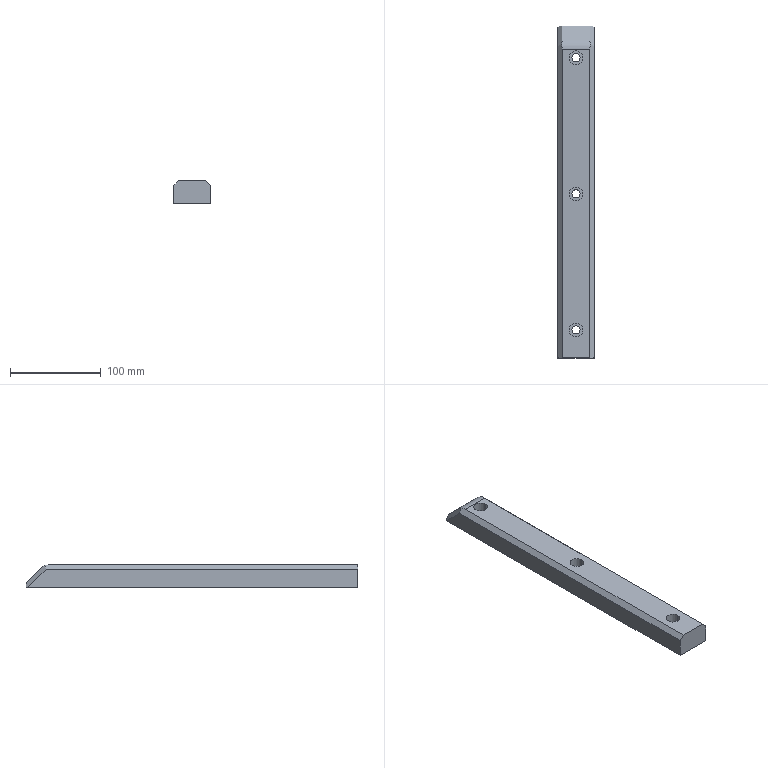Part | SolidWorks | features Chamfer 4, Fillet 4, ICE 3, HoleWzd 2, Extrusion 1 | 1 solid | 27 faces | box 40 x 366 x 25 mm | volume 339646 mm3 | plane 14 | cylinder 13 | commonest cylinder face diameters 9 x6 15 x6 30 x1
STEP:
#1=CARTESIAN_POINT('',(-4.5,-152.,0.));
#2=VERTEX_POINT('',#1);
#3=CARTESIAN_POINT('',(4.5,-152.,0.));
#4=VERTEX_POINT('',#3);
#5=CARTESIAN_POINT('',(0.,-152.,0.));
#6=DIRECTION('',(0.,0.,1.));
#7=DIRECTION('',(1.,0.,0.));
#8=AXIS2_PLACEMENT_3D('',#5,#6,#7);
#9=CIRCLE('',#8,4.5);
#10=EDGE_CURVE('',#2,#4,#9,.T.);
#11=ORIENTED_EDGE('',*,*,#10,.F.);
#12=CARTESIAN_POINT('',(-4.5,-152.,13.));
#13=VERTEX_POINT('',#12);
#14=CARTESIAN_POINT('',(-4.5,-152.,23.));
#15=DIRECTION('',(0.,0.,1.));
#16=VECTOR('',#15,1000.);
#17=LINE('',#14,#16);
#18=EDGE_CURVE('',#2,#13,#17,.T.);
#19=ORIENTED_EDGE('',*,*,#18,.T.);
#20=CARTESIAN_POINT('',(4.5,-152.,13.));
#21=VERTEX_POINT('',#20);
#22=CARTESIAN_POINT('',(0.,-152.,13.));
#23=DIRECTION('',(0.,0.,1.));
#24=DIRECTION('',(1.,0.,0.));
#25=AXIS2_PLACEMENT_3D('',#22,#23,#24);
#26=CIRCLE('',#25,4.5);
#27=EDGE_CURVE('',#13,#21,#26,.T.);
#28=ORIENTED_EDGE('',*,*,#27,.T.);
#29=CARTESIAN_POINT('',(4.5,-152.,23.));
#30=DIRECTION('',(0.,0.,1.));
#31=VECTOR('',#30,1000.);
#32=LINE('',#29,#31);
#33=EDGE_CURVE('',#4,#21,#32,.T.);
#34=ORIENTED_EDGE('',*,*,#33,.F.);
#35=EDGE_LOOP('',(#11,#19,#28,#34));
#36=FACE_OUTER_BOUND('',#35,.T.);
#37=CARTESIAN_POINT('',(0.,-152.,23.));
#38=DIRECTION('',(0.,0.,1.));
#39=DIRECTION('',(1.,0.,0.));
#40=AXIS2_PLACEMENT_3D('',#37,#38,#39);
#41=CYLINDRICAL_SURFACE('',#40,4.5);
#42=ADVANCED_FACE('',(#36),#41,.F.);
#43=CARTESIAN_POINT('',(-4.5,-2.,0.));
#44=VERTEX_POINT('',#43);
#45=CARTESIAN_POINT('',(4.5,-2.,0.));
#46=VERTEX_POINT('',#45);
#47=CARTESIAN_POINT('',(0.,-2.,0.));
#48=DIRECTION('',(0.,0.,1.));
#49=DIRECTION('',(1.,0.,0.));
#50=AXIS2_PLACEMENT_3D('',#47,#48,#49);
#51=CIRCLE('',#50,4.5);
#52=EDGE_CURVE('',#44,#46,#51,.T.);
#53=ORIENTED_EDGE('',*,*,#52,.F.);
#54=CARTESIAN_POINT('',(-4.5,-2.,13.));
#55=VERTEX_POINT('',#54);
#56=CARTESIAN_POINT('',(-4.5,-2.,23.));
#57=DIRECTION('',(0.,0.,1.));
#58=VECTOR('',#57,1000.);
#59=LINE('',#56,#58);
#60=EDGE_CURVE('',#44,#55,#59,.T.);
#61=ORIENTED_EDGE('',*,*,#60,.T.);
#62=CARTESIAN_POINT('',(4.5,-2.,13.));
#63=VERTEX_POINT('',#62);
#64=CARTESIAN_POINT('',(0.,-2.,13.));
#65=DIRECTION('',(0.,0.,1.));
#66=DIRECTION('',(1.,0.,0.));
#67=AXIS2_PLACEMENT_3D('',#64,#65,#66);
#68=CIRCLE('',#67,4.5);
#69=EDGE_CURVE('',#55,#63,#68,.T.);
#70=ORIENTED_EDGE('',*,*,#69,.T.);
#71=CARTESIAN_POINT('',(4.5,-2.,23.));
#72=DIRECTION('',(0.,0.,1.));
#73=VECTOR('',#72,1000.);
#74=LINE('',#71,#73);
#75=EDGE_CURVE('',#46,#63,#74,.T.);
#76=ORIENTED_EDGE('',*,*,#75,.F.);
#77=EDGE_LOOP('',(#53,#61,#70,#76));
#78=FACE_OUTER_BOUND('',#77,.T.);
#79=CARTESIAN_POINT('',(0.,-2.,23.));
#80=DIRECTION('',(0.,0.,1.));
#81=DIRECTION('',(1.,0.,0.));
#82=AXIS2_PLACEMENT_3D('',#79,#80,#81);
#83=CYLINDRICAL_SURFACE('',#82,4.5);
#84=ADVANCED_FACE('',(#78),#83,.F.);
#85=CARTESIAN_POINT('',(-4.5,148.,0.));
#86=VERTEX_POINT('',#85);
#87=CARTESIAN_POINT('',(4.5,148.,0.));
#88=VERTEX_POINT('',#87);
#89=CARTESIAN_POINT('',(0.,148.,0.));
#90=DIRECTION('',(0.,0.,1.));
#91=DIRECTION('',(1.,0.,0.));
#92=AXIS2_PLACEMENT_3D('',#89,#90,#91);
#93=CIRCLE('',#92,4.5);
#94=EDGE_CURVE('',#86,#88,#93,.T.);
#95=ORIENTED_EDGE('',*,*,#94,.F.);
#96=CARTESIAN_POINT('',(-4.5,148.,13.));
#97=VERTEX_POINT('',#96);
#98=CARTESIAN_POINT('',(-4.5,148.,23.));
#99=DIRECTION('',(0.,0.,1.));
#100=VECTOR('',#99,1000.);
#101=LINE('',#98,#100);
#102=EDGE_CURVE('',#86,#97,#101,.T.);
#103=ORIENTED_EDGE('',*,*,#102,.T.);
#104=CARTESIAN_POINT('',(4.5,148.,13.));
#105=VERTEX_POINT('',#104);
#106=CARTESIAN_POINT('',(0.,148.,13.));
#107=DIRECTION('',(0.,0.,1.));
#108=DIRECTION('',(1.,0.,0.));
#109=AXIS2_PLACEMENT_3D('',#106,#107,#108);
#110=CIRCLE('',#109,4.5);
#111=EDGE_CURVE('',#97,#105,#110,.T.);
#112=ORIENTED_EDGE('',*,*,#111,.T.);
#113=CARTESIAN_POINT('',(4.5,148.,23.));
#114=DIRECTION('',(0.,0.,1.));
#115=VECTOR('',#114,1000.);
#116=LINE('',#113,#115);
#117=EDGE_CURVE('',#88,#105,#116,.T.);
#118=ORIENTED_EDGE('',*,*,#117,.F.);
#119=EDGE_LOOP('',(#95,#103,#112,#118));
#120=FACE_OUTER_BOUND('',#119,.T.);
#121=CARTESIAN_POINT('',(0.,148.,23.));
#122=DIRECTION('',(0.,0.,1.));
#123=DIRECTION('',(1.,0.,0.));
#124=AXIS2_PLACEMENT_3D('',#121,#122,#123);
#125=CYLINDRICAL_SURFACE('',#124,4.5);
#126=ADVANCED_FACE('',(#120),#125,.F.);
#127=CARTESIAN_POINT('',(-7.5,-152.,13.));
#128=VERTEX_POINT('',#127);
#129=CARTESIAN_POINT('',(7.5,-152.,13.));
#130=VERTEX_POINT('',#129);
#131=CARTESIAN_POINT('',(0.,-152.,13.));
#132=DIRECTION('',(0.,0.,1.));
#133=DIRECTION('',(1.,0.,0.));
#134=AXIS2_PLACEMENT_3D('',#131,#132,#133);
#135=CIRCLE('',#134,7.5);
#136=EDGE_CURVE('',#128,#130,#135,.T.);
#137=ORIENTED_EDGE('',*,*,#136,.F.);
#138=CARTESIAN_POINT('',(-7.5,-152.,25.));
#139=VERTEX_POINT('',#138);
#140=CARTESIAN_POINT('',(-7.5,-152.,23.));
#141=DIRECTION('',(0.,0.,1.));
#142=VECTOR('',#141,1000.);
#143=LINE('',#140,#142);
#144=EDGE_CURVE('',#128,#139,#143,.T.);
#145=ORIENTED_EDGE('',*,*,#144,.T.);
#146=CARTESIAN_POINT('',(7.5,-152.,25.));
#147=VERTEX_POINT('',#146);
#148=CARTESIAN_POINT('',(0.,-152.,25.));
#149=DIRECTION('',(0.,0.,1.));
#150=DIRECTION('',(1.,0.,0.));
#151=AXIS2_PLACEMENT_3D('',#148,#149,#150);
#152=CIRCLE('',#151,7.5);
#153=EDGE_CURVE('',#139,#147,#152,.T.);
#154=ORIENTED_EDGE('',*,*,#153,.T.);
#155=CARTESIAN_POINT('',(7.5,-152.,23.));
#156=DIRECTION('',(0.,0.,1.));
#157=VECTOR('',#156,1000.);
#158=LINE('',#155,#157);
#159=EDGE_CURVE('',#130,#147,#158,.T.);
#160=ORIENTED_EDGE('',*,*,#159,.F.);
#161=EDGE_LOOP('',(#137,#145,#154,#160));
#162=FACE_OUTER_BOUND('',#161,.T.);
#163=CARTESIAN_POINT('',(0.,-152.,23.));
#164=DIRECTION('',(0.,0.,1.));
#165=DIRECTION('',(1.,0.,0.));
#166=AXIS2_PLACEMENT_3D('',#163,#164,#165);
#167=CYLINDRICAL_SURFACE('',#166,7.5);
#168=ADVANCED_FACE('',(#162),#167,.F.);
#169=CARTESIAN_POINT('',(-7.5,-2.,13.));
#170=VERTEX_POINT('',#169);
#171=CARTESIAN_POINT('',(7.5,-2.,13.));
#172=VERTEX_POINT('',#171);
#173=CARTESIAN_POINT('',(0.,-2.,13.));
#174=DIRECTION('',(0.,0.,1.));
#175=DIRECTION('',(1.,0.,0.));
#176=AXIS2_PLACEMENT_3D('',#173,#174,#175);
#177=CIRCLE('',#176,7.5);
#178=EDGE_CURVE('',#170,#172,#177,.T.);
#179=ORIENTED_EDGE('',*,*,#178,.F.);
#180=CARTESIAN_POINT('',(-7.5,-2.,25.));
#181=VERTEX_POINT('',#180);
#182=CARTESIAN_POINT('',(-7.5,-2.,23.));
#183=DIRECTION('',(0.,0.,1.));
#184=VECTOR('',#183,1000.);
#185=LINE('',#182,#184);
#186=EDGE_CURVE('',#170,#181,#185,.T.);
#187=ORIENTED_EDGE('',*,*,#186,.T.);
#188=CARTESIAN_POINT('',(7.5,-2.,25.));
#189=VERTEX_POINT('',#188);
#190=CARTESIAN_POINT('',(0.,-2.,25.));
#191=DIRECTION('',(0.,0.,1.));
#192=DIRECTION('',(1.,0.,0.));
#193=AXIS2_PLACEMENT_3D('',#190,#191,#192);
#194=CIRCLE('',#193,7.5);
#195=EDGE_CURVE('',#181,#189,#194,.T.);
#196=ORIENTED_EDGE('',*,*,#195,.T.);
#197=CARTESIAN_POINT('',(7.5,-2.,23.));
#198=DIRECTION('',(0.,0.,1.));
#199=VECTOR('',#198,1000.);
#200=LINE('',#197,#199);
#201=EDGE_CURVE('',#172,#189,#200,.T.);
#202=ORIENTED_EDGE('',*,*,#201,.F.);
#203=EDGE_LOOP('',(#179,#187,#196,#202));
#204=FACE_OUTER_BOUND('',#203,.T.);
#205=CARTESIAN_POINT('',(0.,-2.,23.));
#206=DIRECTION('',(0.,0.,1.));
#207=DIRECTION('',(1.,0.,0.));
#208=AXIS2_PLACEMENT_3D('',#205,#206,#207);
#209=CYLINDRICAL_SURFACE('',#208,7.5);
#210=ADVANCED_FACE('',(#204),#209,.F.);
#211=CARTESIAN_POINT('',(-7.5,148.,13.));
#212=VERTEX_POINT('',#211);
#213=CARTESIAN_POINT('',(7.5,148.,13.));
#214=VERTEX_POINT('',#213);
#215=CARTESIAN_POINT('',(0.,148.,13.));
#216=DIRECTION('',(0.,0.,1.));
#217=DIRECTION('',(1.,0.,0.));
#218=AXIS2_PLACEMENT_3D('',#215,#216,#217);
#219=CIRCLE('',#218,7.5);
#220=EDGE_CURVE('',#212,#214,#219,.T.);
#221=ORIENTED_EDGE('',*,*,#220,.F.);
#222=CARTESIAN_POINT('',(-7.5,148.,25.));
#223=VERTEX_POINT('',#222);
#224=CARTESIAN_POINT('',(-7.5,148.,23.));
#225=DIRECTION('',(0.,0.,1.));
#226=VECTOR('',#225,1000.);
#227=LINE('',#224,#226);
#228=EDGE_CURVE('',#212,#223,#227,.T.);
#229=ORIENTED_EDGE('',*,*,#228,.T.);
#230=CARTESIAN_POINT('',(7.5,148.,25.));
#231=VERTEX_POINT('',#230);
#232=CARTESIAN_POINT('',(0.,148.,25.));
#233=DIRECTION('',(0.,0.,1.));
#234=DIRECTION('',(1.,0.,0.));
#235=AXIS2_PLACEMENT_3D('',#232,#233,#234);
#236=CIRCLE('',#235,7.5);
#237=EDGE_CURVE('',#223,#231,#236,.T.);
#238=ORIENTED_EDGE('',*,*,#237,.T.);
#239=CARTESIAN_POINT('',(7.5,148.,23.));
#240=DIRECTION('',(0.,0.,1.));
#241=VECTOR('',#240,1000.);
#242=LINE('',#239,#241);
#243=EDGE_CURVE('',#214,#231,#242,.T.);
#244=ORIENTED_EDGE('',*,*,#243,.F.);
#245=EDGE_LOOP('',(#221,#229,#238,#244));
#246=FACE_OUTER_BOUND('',#245,.T.);
#247=CARTESIAN_POINT('',(0.,148.,23.));
#248=DIRECTION('',(0.,0.,1.));
#249=DIRECTION('',(1.,0.,0.));
#250=AXIS2_PLACEMENT_3D('',#247,#248,#249);
#251=CYLINDRICAL_SURFACE('',#250,7.5);
#252=ADVANCED_FACE('',(#246),#251,.F.);
#253=CARTESIAN_POINT('',(20.,-183.,0.));
#254=VERTEX_POINT('',#253);
#255=CARTESIAN_POINT('',(20.,180.929,0.));
#256=VERTEX_POINT('',#255);
#257=CARTESIAN_POINT('',(20.,183.,0.));
#258=DIRECTION('',(0.,1.,0.));
#259=VECTOR('',#258,1000.);
#260=LINE('',#257,#259);
#261=EDGE_CURVE('',#254,#256,#260,.T.);
#262=ORIENTED_EDGE('',*,*,#261,.T.);
#263=CARTESIAN_POINT('',(20.,160.929,20.));
#264=VERTEX_POINT('',#263);
#265=CARTESIAN_POINT('',(20.,164.464,16.464));
#266=DIRECTION('',(0.,-0.7071,0.7071));
#267=VECTOR('',#266,1000.);
#268=LINE('',#265,#267);
#269=EDGE_CURVE('',#256,#264,#268,.T.);
#270=ORIENTED_EDGE('',*,*,#269,.T.);
#271=CARTESIAN_POINT('',(20.,-183.,20.));
#272=VERTEX_POINT('',#271);
#273=CARTESIAN_POINT('',(20.,-183.,20.));
#274=DIRECTION('',(0.,-1.,0.));
#275=VECTOR('',#274,1000.);
#276=LINE('',#273,#275);
#277=EDGE_CURVE('',#264,#272,#276,.T.);
#278=ORIENTED_EDGE('',*,*,#277,.T.);
#279=CARTESIAN_POINT('',(20.,-183.,25.));
#280=DIRECTION('',(0.,0.,-1.));
#281=VECTOR('',#280,1000.);
#282=LINE('',#279,#281);
#283=EDGE_CURVE('',#272,#254,#282,.T.);
#284=ORIENTED_EDGE('',*,*,#283,.T.);
#285=EDGE_LOOP('',(#262,#270,#278,#284));
#286=FACE_OUTER_BOUND('',#285,.T.);
#287=CARTESIAN_POINT('',(20.,183.,25.));
#288=DIRECTION('',(-1.,0.,0.));
#289=DIRECTION('',(0.,-1.,0.));
#290=AXIS2_PLACEMENT_3D('',#287,#288,#289);
#291=PLANE('',#290);
#292=ADVANCED_FACE('',(#286),#291,.F.);
#293=CARTESIAN_POINT('',(-15.,183.,5.));
#294=VERTEX_POINT('',#293);
#295=CARTESIAN_POINT('',(15.,183.,5.));
#296=VERTEX_POINT('',#295);
#297=CARTESIAN_POINT('',(20.,183.,5.));
#298=DIRECTION('',(1.,0.,0.));
#299=VECTOR('',#298,1000.);
#300=LINE('',#297,#299);
#301=EDGE_CURVE('',#294,#296,#300,.T.);
#302=ORIENTED_EDGE('',*,*,#301,.T.);
#303=CARTESIAN_POINT('',(18.536,183.,0.));
#304=VERTEX_POINT('',#303);
#305=CARTESIAN_POINT('',(13.619,183.,6.953));
#306=DIRECTION('',(0.5774,0.,-0.8165));
#307=VECTOR('',#306,1000.);
#308=LINE('',#305,#307);
#309=EDGE_CURVE('',#296,#304,#308,.T.);
#310=ORIENTED_EDGE('',*,*,#309,.T.);
#311=CARTESIAN_POINT('',(-18.536,183.,0.));
#312=VERTEX_POINT('',#311);
#313=CARTESIAN_POINT('',(-20.,183.,0.));
#314=DIRECTION('',(-1.,0.,0.));
#315=VECTOR('',#314,1000.);
#316=LINE('',#313,#315);
#317=EDGE_CURVE('',#304,#312,#316,.T.);
#318=ORIENTED_EDGE('',*,*,#317,.T.);
#319=CARTESIAN_POINT('',(-13.619,183.,6.953));
#320=DIRECTION('',(0.5774,0.,0.8165));
#321=VECTOR('',#320,1000.);
#322=LINE('',#319,#321);
#323=EDGE_CURVE('',#312,#294,#322,.T.);
#324=ORIENTED_EDGE('',*,*,#323,.T.);
#325=EDGE_LOOP('',(#302,#310,#318,#324));
#326=FACE_OUTER_BOUND('',#325,.T.);
#327=CARTESIAN_POINT('',(-20.,183.,25.));
#328=DIRECTION('',(0.,-1.,0.));
#329=DIRECTION('',(0.,0.,-1.));
#330=AXIS2_PLACEMENT_3D('',#327,#328,#329);
#331=PLANE('',#330);
#332=ADVANCED_FACE('',(#326),#331,.F.);
#333=CARTESIAN_POINT('',(-20.,-183.,20.));
#334=VERTEX_POINT('',#333);
#335=CARTESIAN_POINT('',(-20.,160.929,20.));
#336=VERTEX_POINT('',#335);
#337=CARTESIAN_POINT('',(-20.,163.,20.));
#338=DIRECTION('',(0.,1.,0.));
#339=VECTOR('',#338,1000.);
#340=LINE('',#337,#339);
#341=EDGE_CURVE('',#334,#336,#340,.T.);
#342=ORIENTED_EDGE('',*,*,#341,.T.);
#343=CARTESIAN_POINT('',(-20.,180.929,0.));
#344=VERTEX_POINT('',#343);
#345=CARTESIAN_POINT('',(-20.,179.464,1.464));
#346=DIRECTION('',(0.,0.7071,-0.7071));
#347=VECTOR('',#346,1000.);
#348=LINE('',#345,#347);
#349=EDGE_CURVE('',#336,#344,#348,.T.);
#350=ORIENTED_EDGE('',*,*,#349,.T.);
#351=CARTESIAN_POINT('',(-20.,-183.,0.));
#352=VERTEX_POINT('',#351);
#353=CARTESIAN_POINT('',(-20.,183.,0.));
#354=DIRECTION('',(0.,-1.,0.));
#355=VECTOR('',#354,1000.);
#356=LINE('',#353,#355);
#357=EDGE_CURVE('',#344,#352,#356,.T.);
#358=ORIENTED_EDGE('',*,*,#357,.T.);
#359=CARTESIAN_POINT('',(-20.,-183.,25.));
#360=DIRECTION('',(0.,0.,-1.));
#361=VECTOR('',#360,1000.);
#362=LINE('',#359,#361);
#363=EDGE_CURVE('',#334,#352,#362,.T.);
#364=ORIENTED_EDGE('',*,*,#363,.F.);
#365=EDGE_LOOP('',(#342,#350,#358,#364));
#366=FACE_OUTER_BOUND('',#365,.T.);
#367=CARTESIAN_POINT('',(-20.,183.,25.));
#368=DIRECTION('',(1.,0.,0.));
#369=DIRECTION('',(0.,1.,0.));
#370=AXIS2_PLACEMENT_3D('',#367,#368,#369);
#371=PLANE('',#370);
#372=ADVANCED_FACE('',(#366),#371,.F.);
#373=ORIENTED_EDGE('',*,*,#283,.F.);
#374=CARTESIAN_POINT('',(15.,-183.,25.));
#375=VERTEX_POINT('',#374);
#376=CARTESIAN_POINT('',(15.,-183.,25.));
#377=DIRECTION('',(-0.7071,0.,0.7071));
#378=VECTOR('',#377,1000.);
#379=LINE('',#376,#378);
#380=EDGE_CURVE('',#272,#375,#379,.T.);
#381=ORIENTED_EDGE('',*,*,#380,.T.);
#382=CARTESIAN_POINT('',(-15.,-183.,25.));
#383=VERTEX_POINT('',#382);
#384=CARTESIAN_POINT('',(-20.,-183.,25.));
#385=DIRECTION('',(1.,0.,0.));
#386=VECTOR('',#385,1000.);
#387=LINE('',#384,#386);
#388=EDGE_CURVE('',#383,#375,#387,.T.);
#389=ORIENTED_EDGE('',*,*,#388,.F.);
#390=CARTESIAN_POINT('',(-15.,-183.,25.));
#391=DIRECTION('',(-0.7071,0.,-0.7071));
#392=VECTOR('',#391,1000.);
#393=LINE('',#390,#392);
#394=EDGE_CURVE('',#383,#334,#393,.T.);
#395=ORIENTED_EDGE('',*,*,#394,.T.);
#396=ORIENTED_EDGE('',*,*,#363,.T.);
#397=CARTESIAN_POINT('',(-20.,-183.,0.));
#398=DIRECTION('',(1.,0.,0.));
#399=VECTOR('',#398,1000.);
#400=LINE('',#397,#399);
#401=EDGE_CURVE('',#352,#254,#400,.T.);
#402=ORIENTED_EDGE('',*,*,#401,.T.);
#403=EDGE_LOOP('',(#373,#381,#389,#395,#396,#402));
#404=FACE_OUTER_BOUND('',#403,.T.);
#405=CARTESIAN_POINT('',(-20.,-183.,25.));
#406=DIRECTION('',(0.,1.,0.));
#407=DIRECTION('',(0.,0.,1.));
#408=AXIS2_PLACEMENT_3D('',#405,#406,#407);
#409=PLANE('',#408);
#410=ADVANCED_FACE('',(#404),#409,.F.);
#411=CARTESIAN_POINT('',(0.,-152.,25.));
#412=DIRECTION('',(0.,0.,1.));
#413=DIRECTION('',(1.,0.,0.));
#414=AXIS2_PLACEMENT_3D('',#411,#412,#413);
#415=CIRCLE('',#414,7.5);
#416=EDGE_CURVE('',#147,#139,#415,.T.);
#417=ORIENTED_EDGE('',*,*,#416,.F.);
#418=ORIENTED_EDGE('',*,*,#153,.F.);
#419=EDGE_LOOP('',(#417,#418));
#420=FACE_BOUND('',#419,.T.);
#421=CARTESIAN_POINT('',(0.,-2.,25.));
#422=DIRECTION('',(0.,0.,1.));
#423=DIRECTION('',(1.,0.,0.));
#424=AXIS2_PLACEMENT_3D('',#421,#422,#423);
#425=CIRCLE('',#424,7.5);
#426=EDGE_CURVE('',#189,#181,#425,.T.);
#427=ORIENTED_EDGE('',*,*,#426,.F.);
#428=ORIENTED_EDGE('',*,*,#195,.F.);
#429=EDGE_LOOP('',(#427,#428));
#430=FACE_BOUND('',#429,.T.);
#431=CARTESIAN_POINT('',(0.,148.,25.));
#432=DIRECTION('',(0.,0.,1.));
#433=DIRECTION('',(1.,0.,0.));
#434=AXIS2_PLACEMENT_3D('',#431,#432,#433);
#435=CIRCLE('',#434,7.5);
#436=EDGE_CURVE('',#231,#223,#435,.T.);
#437=ORIENTED_EDGE('',*,*,#436,.F.);
#438=ORIENTED_EDGE('',*,*,#237,.F.);
#439=EDGE_LOOP('',(#437,#438));
#440=FACE_BOUND('',#439,.T.);
#441=CARTESIAN_POINT('',(15.,156.787,25.));
#442=VERTEX_POINT('',#441);
#443=CARTESIAN_POINT('',(15.,163.,25.));
#444=DIRECTION('',(0.,1.,0.));
#445=VECTOR('',#444,1000.);
#446=LINE('',#443,#445);
#447=EDGE_CURVE('',#375,#442,#446,.T.);
#448=ORIENTED_EDGE('',*,*,#447,.T.);
#449=CARTESIAN_POINT('',(-15.,156.787,25.));
#450=VERTEX_POINT('',#449);
#451=CARTESIAN_POINT('',(0.,156.787,25.));
#452=DIRECTION('',(-1.,0.,0.));
#453=VECTOR('',#452,1000.);
#454=LINE('',#451,#453);
#455=EDGE_CURVE('',#442,#450,#454,.T.);
#456=ORIENTED_EDGE('',*,*,#455,.T.);
#457=CARTESIAN_POINT('',(-15.,-183.,25.));
#458=DIRECTION('',(0.,-1.,0.));
#459=VECTOR('',#458,1000.);
#460=LINE('',#457,#459);
#461=EDGE_CURVE('',#450,#383,#460,.T.);
#462=ORIENTED_EDGE('',*,*,#461,.T.);
#463=ORIENTED_EDGE('',*,*,#388,.T.);
#464=EDGE_LOOP('',(#448,#456,#462,#463));
#465=FACE_OUTER_BOUND('',#464,.T.);
#466=CARTESIAN_POINT('',(0.,0.,25.));
#467=DIRECTION('',(0.,0.,1.));
#468=DIRECTION('',(1.,0.,0.));
#469=AXIS2_PLACEMENT_3D('',#466,#467,#468);
#470=PLANE('',#469);
#471=ADVANCED_FACE('',(#420,#430,#440,#465),#470,.T.);
#472=CARTESIAN_POINT('',(0.,-152.,0.));
#473=DIRECTION('',(0.,0.,1.));
#474=DIRECTION('',(1.,0.,0.));
#475=AXIS2_PLACEMENT_3D('',#472,#473,#474);
#476=CIRCLE('',#475,4.5);
#477=EDGE_CURVE('',#4,#2,#476,.T.);
#478=ORIENTED_EDGE('',*,*,#477,.T.);
#479=ORIENTED_EDGE('',*,*,#10,.T.);
#480=EDGE_LOOP('',(#478,#479));
#481=FACE_BOUND('',#480,.T.);
#482=CARTESIAN_POINT('',(0.,-2.,0.));
#483=DIRECTION('',(0.,0.,1.));
#484=DIRECTION('',(1.,0.,0.));
#485=AXIS2_PLACEMENT_3D('',#482,#483,#484);
#486=CIRCLE('',#485,4.5);
#487=EDGE_CURVE('',#46,#44,#486,.T.);
#488=ORIENTED_EDGE('',*,*,#487,.T.);
#489=ORIENTED_EDGE('',*,*,#52,.T.);
#490=EDGE_LOOP('',(#488,#489));
#491=FACE_BOUND('',#490,.T.);
#492=CARTESIAN_POINT('',(0.,148.,0.));
#493=DIRECTION('',(0.,0.,1.));
#494=DIRECTION('',(1.,0.,0.));
#495=AXIS2_PLACEMENT_3D('',#492,#493,#494);
#496=CIRCLE('',#495,4.5);
#497=EDGE_CURVE('',#88,#86,#496,.T.);
#498=ORIENTED_EDGE('',*,*,#497,.T.);
#499=ORIENTED_EDGE('',*,*,#94,.T.);
#500=EDGE_LOOP('',(#498,#499));
#501=FACE_BOUND('',#500,.T.);
#502=ORIENTED_EDGE('',*,*,#317,.F.);
#503=CARTESIAN_POINT('',(25.404,173.286,0.));
#504=DIRECTION('',(0.5774,-0.8165,0.));
#505=VECTOR('',#504,1000.);
#506=LINE('',#503,#505);
#507=EDGE_CURVE('',#304,#256,#506,.T.);
#508=ORIENTED_EDGE('',*,*,#507,.T.);
#509=ORIENTED_EDGE('',*,*,#261,.F.);
#510=ORIENTED_EDGE('',*,*,#401,.F.);
#511=ORIENTED_EDGE('',*,*,#357,.F.);
#512=CARTESIAN_POINT('',(-25.404,173.286,0.));
#513=DIRECTION('',(0.5774,0.8165,0.));
#514=VECTOR('',#513,1000.);
#515=LINE('',#512,#514);
#516=EDGE_CURVE('',#344,#312,#515,.T.);
#517=ORIENTED_EDGE('',*,*,#516,.T.);
#518=EDGE_LOOP('',(#502,#508,#509,#510,#511,#517));
#519=FACE_OUTER_BOUND('',#518,.T.);
#520=CARTESIAN_POINT('',(0.,0.,0.));
#521=DIRECTION('',(0.,0.,1.));
#522=DIRECTION('',(1.,0.,0.));
#523=AXIS2_PLACEMENT_3D('',#520,#521,#522);
#524=PLANE('',#523);
#525=ADVANCED_FACE('',(#481,#491,#501,#519),#524,.F.);
#526=CARTESIAN_POINT('',(-15.,167.393,20.607));
#527=VERTEX_POINT('',#526);
#528=CARTESIAN_POINT('',(-15.,168.,20.));
#529=DIRECTION('',(0.,-0.7071,0.7071));
#530=VECTOR('',#529,1000.);
#531=LINE('',#528,#530);
#532=EDGE_CURVE('',#294,#527,#531,.T.);
#533=ORIENTED_EDGE('',*,*,#532,.T.);
#534=CARTESIAN_POINT('',(15.,167.393,20.607));
#535=VERTEX_POINT('',#534);
#536=CARTESIAN_POINT('',(0.,167.393,20.607));
#537=DIRECTION('',(1.,0.,0.));
#538=VECTOR('',#537,1000.);
#539=LINE('',#536,#538);
#540=EDGE_CURVE('',#527,#535,#539,.T.);
#541=ORIENTED_EDGE('',*,*,#540,.T.);
#542=CARTESIAN_POINT('',(15.,183.,5.));
#543=DIRECTION('',(0.,0.7071,-0.7071));
#544=VECTOR('',#543,1000.);
#545=LINE('',#542,#544);
#546=EDGE_CURVE('',#535,#296,#545,.T.);
#547=ORIENTED_EDGE('',*,*,#546,.T.);
#548=ORIENTED_EDGE('',*,*,#301,.F.);
#549=EDGE_LOOP('',(#533,#541,#547,#548));
#550=FACE_OUTER_BOUND('',#549,.T.);
#551=CARTESIAN_POINT('',(0.,163.,25.));
#552=DIRECTION('',(0.,0.7071,0.7071));
#553=DIRECTION('',(1.,0.,0.));
#554=AXIS2_PLACEMENT_3D('',#551,#552,#553);
#555=PLANE('',#554);
#556=ADVANCED_FACE('',(#550),#555,.T.);
#557=ORIENTED_EDGE('',*,*,#228,.F.);
#558=CARTESIAN_POINT('',(0.,148.,13.));
#559=DIRECTION('',(0.,0.,1.));
#560=DIRECTION('',(1.,0.,0.));
#561=AXIS2_PLACEMENT_3D('',#558,#559,#560);
#562=CIRCLE('',#561,7.5);
#563=EDGE_CURVE('',#214,#212,#562,.T.);
#564=ORIENTED_EDGE('',*,*,#563,.F.);
#565=ORIENTED_EDGE('',*,*,#243,.T.);
#566=ORIENTED_EDGE('',*,*,#436,.T.);
#567=EDGE_LOOP('',(#557,#564,#565,#566));
#568=FACE_OUTER_BOUND('',#567,.T.);
#569=CARTESIAN_POINT('',(0.,148.,23.));
#570=DIRECTION('',(0.,0.,1.));
#571=DIRECTION('',(1.,0.,0.));
#572=AXIS2_PLACEMENT_3D('',#569,#570,#571);
#573=CYLINDRICAL_SURFACE('',#572,7.5);
#574=ADVANCED_FACE('',(#568),#573,.F.);
#575=ORIENTED_EDGE('',*,*,#186,.F.);
#576=CARTESIAN_POINT('',(0.,-2.,13.));
#577=DIRECTION('',(0.,0.,1.));
#578=DIRECTION('',(1.,0.,0.));
#579=AXIS2_PLACEMENT_3D('',#576,#577,#578);
#580=CIRCLE('',#579,7.5);
#581=EDGE_CURVE('',#172,#170,#580,.T.);
#582=ORIENTED_EDGE('',*,*,#581,.F.);
#583=ORIENTED_EDGE('',*,*,#201,.T.);
#584=ORIENTED_EDGE('',*,*,#426,.T.);
#585=EDGE_LOOP('',(#575,#582,#583,#584));
#586=FACE_OUTER_BOUND('',#585,.T.);
#587=CARTESIAN_POINT('',(0.,-2.,23.));
#588=DIRECTION('',(0.,0.,1.));
#589=DIRECTION('',(1.,0.,0.));
#590=AXIS2_PLACEMENT_3D('',#587,#588,#589);
#591=CYLINDRICAL_SURFACE('',#590,7.5);
#592=ADVANCED_FACE('',(#586),#591,.F.);
#593=ORIENTED_EDGE('',*,*,#144,.F.);
#594=CARTESIAN_POINT('',(0.,-152.,13.));
#595=DIRECTION('',(0.,0.,1.));
#596=DIRECTION('',(1.,0.,0.));
#597=AXIS2_PLACEMENT_3D('',#594,#595,#596);
#598=CIRCLE('',#597,7.5);
#599=EDGE_CURVE('',#130,#128,#598,.T.);
#600=ORIENTED_EDGE('',*,*,#599,.F.);
#601=ORIENTED_EDGE('',*,*,#159,.T.);
#602=ORIENTED_EDGE('',*,*,#416,.T.);
#603=EDGE_LOOP('',(#593,#600,#601,#602));
#604=FACE_OUTER_BOUND('',#603,.T.);
#605=CARTESIAN_POINT('',(0.,-152.,23.));
#606=DIRECTION('',(0.,0.,1.));
#607=DIRECTION('',(1.,0.,0.));
#608=AXIS2_PLACEMENT_3D('',#605,#606,#607);
#609=CYLINDRICAL_SURFACE('',#608,7.5);
#610=ADVANCED_FACE('',(#604),#609,.F.);
#611=ORIENTED_EDGE('',*,*,#102,.F.);
#612=ORIENTED_EDGE('',*,*,#497,.F.);
#613=ORIENTED_EDGE('',*,*,#117,.T.);
#614=CARTESIAN_POINT('',(0.,148.,13.));
#615=DIRECTION('',(0.,0.,1.));
#616=DIRECTION('',(1.,0.,0.));
#617=AXIS2_PLACEMENT_3D('',#614,#615,#616);
#618=CIRCLE('',#617,4.5);
#619=EDGE_CURVE('',#105,#97,#618,.T.);
#620=ORIENTED_EDGE('',*,*,#619,.T.);
#621=EDGE_LOOP('',(#611,#612,#613,#620));
#622=FACE_OUTER_BOUND('',#621,.T.);
#623=CARTESIAN_POINT('',(0.,148.,23.));
#624=DIRECTION('',(0.,0.,1.));
#625=DIRECTION('',(1.,0.,0.));
#626=AXIS2_PLACEMENT_3D('',#623,#624,#625);
#627=CYLINDRICAL_SURFACE('',#626,4.5);
#628=ADVANCED_FACE('',(#622),#627,.F.);
#629=ORIENTED_EDGE('',*,*,#619,.F.);
#630=ORIENTED_EDGE('',*,*,#111,.F.);
#631=EDGE_LOOP('',(#629,#630));
#632=FACE_BOUND('',#631,.T.);
#633=ORIENTED_EDGE('',*,*,#563,.T.);
#634=ORIENTED_EDGE('',*,*,#220,.T.);
#635=EDGE_LOOP('',(#633,#634));
#636=FACE_OUTER_BOUND('',#635,.T.);
#637=CARTESIAN_POINT('',(4.5,148.,13.));
#638=DIRECTION('',(0.,0.,-1.));
#639=DIRECTION('',(-1.,0.,0.));
#640=AXIS2_PLACEMENT_3D('',#637,#638,#639);
#641=PLANE('',#640);
#642=ADVANCED_FACE('',(#632,#636),#641,.F.);
#643=ORIENTED_EDGE('',*,*,#60,.F.);
#644=ORIENTED_EDGE('',*,*,#487,.F.);
#645=ORIENTED_EDGE('',*,*,#75,.T.);
#646=CARTESIAN_POINT('',(0.,-2.,13.));
#647=DIRECTION('',(0.,0.,1.));
#648=DIRECTION('',(1.,0.,0.));
#649=AXIS2_PLACEMENT_3D('',#646,#647,#648);
#650=CIRCLE('',#649,4.5);
#651=EDGE_CURVE('',#63,#55,#650,.T.);
#652=ORIENTED_EDGE('',*,*,#651,.T.);
#653=EDGE_LOOP('',(#643,#644,#645,#652));
#654=FACE_OUTER_BOUND('',#653,.T.);
#655=CARTESIAN_POINT('',(0.,-2.,23.));
#656=DIRECTION('',(0.,0.,1.));
#657=DIRECTION('',(1.,0.,0.));
#658=AXIS2_PLACEMENT_3D('',#655,#656,#657);
#659=CYLINDRICAL_SURFACE('',#658,4.5);
#660=ADVANCED_FACE('',(#654),#659,.F.);
#661=ORIENTED_EDGE('',*,*,#651,.F.);
#662=ORIENTED_EDGE('',*,*,#69,.F.);
#663=EDGE_LOOP('',(#661,#662));
#664=FACE_BOUND('',#663,.T.);
#665=ORIENTED_EDGE('',*,*,#581,.T.);
#666=ORIENTED_EDGE('',*,*,#178,.T.);
#667=EDGE_LOOP('',(#665,#666));
#668=FACE_OUTER_BOUND('',#667,.T.);
#669=CARTESIAN_POINT('',(4.5,-2.,13.));
#670=DIRECTION('',(0.,0.,-1.));
#671=DIRECTION('',(-1.,0.,0.));
#672=AXIS2_PLACEMENT_3D('',#669,#670,#671);
#673=PLANE('',#672);
#674=ADVANCED_FACE('',(#664,#668),#673,.F.);
#675=ORIENTED_EDGE('',*,*,#18,.F.);
#676=ORIENTED_EDGE('',*,*,#477,.F.);
#677=ORIENTED_EDGE('',*,*,#33,.T.);
#678=CARTESIAN_POINT('',(0.,-152.,13.));
#679=DIRECTION('',(0.,0.,1.));
#680=DIRECTION('',(1.,0.,0.));
#681=AXIS2_PLACEMENT_3D('',#678,#679,#680);
#682=CIRCLE('',#681,4.5);
#683=EDGE_CURVE('',#21,#13,#682,.T.);
#684=ORIENTED_EDGE('',*,*,#683,.T.);
#685=EDGE_LOOP('',(#675,#676,#677,#684));
#686=FACE_OUTER_BOUND('',#685,.T.);
#687=CARTESIAN_POINT('',(0.,-152.,23.));
#688=DIRECTION('',(0.,0.,1.));
#689=DIRECTION('',(1.,0.,0.));
#690=AXIS2_PLACEMENT_3D('',#687,#688,#689);
#691=CYLINDRICAL_SURFACE('',#690,4.5);
#692=ADVANCED_FACE('',(#686),#691,.F.);
#693=ORIENTED_EDGE('',*,*,#683,.F.);
#694=ORIENTED_EDGE('',*,*,#27,.F.);
#695=EDGE_LOOP('',(#693,#694));
#696=FACE_BOUND('',#695,.T.);
#697=ORIENTED_EDGE('',*,*,#599,.T.);
#698=ORIENTED_EDGE('',*,*,#136,.T.);
#699=EDGE_LOOP('',(#697,#698));
#700=FACE_OUTER_BOUND('',#699,.T.);
#701=CARTESIAN_POINT('',(4.5,-152.,13.));
#702=DIRECTION('',(0.,0.,-1.));
#703=DIRECTION('',(-1.,0.,0.));
#704=AXIS2_PLACEMENT_3D('',#701,#702,#703);
#705=PLANE('',#704);
#706=ADVANCED_FACE('',(#696,#700),#705,.F.);
#707=CARTESIAN_POINT('',(16.142,162.527,23.858));
#708=VERTEX_POINT('',#707);
#709=CARTESIAN_POINT('',(46.091,150.122,-6.091));
#710=DIRECTION('',(-0.6786,0.2811,0.6786));
#711=VECTOR('',#710,1000.);
#712=LINE('',#709,#711);
#713=EDGE_CURVE('',#264,#708,#712,.T.);
#714=ORIENTED_EDGE('',*,*,#713,.T.);
#715=CARTESIAN_POINT('',(16.142,162.527,23.858));
#716=CARTESIAN_POINT('',(15.386,160.701,24.614));
#717=CARTESIAN_POINT('',(15.,158.763,25.));
#718=CARTESIAN_POINT('',(15.,156.787,25.));
#719=(BOUNDED_CURVE()B_SPLINE_CURVE(3,(#715,#716,#717,#718),.UNSPECIFIED.,.F.,.T.)B_SPLINE_CURVE_WITH_KNOTS((4,4),(5.89,6.283),.UNSPECIFIED.)CURVE()GEOMETRIC_REPRESENTATION_ITEM()RATIONAL_B_SPLINE_CURVE((1.,0.9872,0.9872,1.))REPRESENTATION_ITEM(''));
#720=EDGE_CURVE('',#708,#442,#719,.T.);
#721=ORIENTED_EDGE('',*,*,#720,.T.);
#722=ORIENTED_EDGE('',*,*,#447,.F.);
#723=ORIENTED_EDGE('',*,*,#380,.F.);
#724=ORIENTED_EDGE('',*,*,#277,.F.);
#725=EDGE_LOOP('',(#714,#721,#722,#723,#724));
#726=FACE_OUTER_BOUND('',#725,.T.);
#727=CARTESIAN_POINT('',(15.,0.,25.));
#728=DIRECTION('',(0.7071,0.,0.7071));
#729=DIRECTION('',(0.,-1.,0.));
#730=AXIS2_PLACEMENT_3D('',#727,#728,#729);
#731=PLANE('',#730);
#732=ADVANCED_FACE('',(#726),#731,.T.);
#733=ORIENTED_EDGE('',*,*,#461,.F.);
#734=CARTESIAN_POINT('',(-16.142,162.527,23.858));
#735=VERTEX_POINT('',#734);
#736=CARTESIAN_POINT('',(-15.,156.787,25.));
#737=CARTESIAN_POINT('',(-15.,158.763,25.));
#738=CARTESIAN_POINT('',(-15.386,160.701,24.614));
#739=CARTESIAN_POINT('',(-16.142,162.527,23.858));
#740=(BOUNDED_CURVE()B_SPLINE_CURVE(3,(#736,#737,#738,#739),.UNSPECIFIED.,.F.,.T.)B_SPLINE_CURVE_WITH_KNOTS((4,4),(3.142,3.534),.UNSPECIFIED.)CURVE()GEOMETRIC_REPRESENTATION_ITEM()RATIONAL_B_SPLINE_CURVE((1.,0.9872,0.9872,1.))REPRESENTATION_ITEM(''));
#741=EDGE_CURVE('',#450,#735,#740,.T.);
#742=ORIENTED_EDGE('',*,*,#741,.T.);
#743=CARTESIAN_POINT('',(-46.091,150.122,-6.091));
#744=DIRECTION('',(-0.6786,-0.2811,-0.6786));
#745=VECTOR('',#744,1000.);
#746=LINE('',#743,#745);
#747=EDGE_CURVE('',#735,#336,#746,.T.);
#748=ORIENTED_EDGE('',*,*,#747,.T.);
#749=ORIENTED_EDGE('',*,*,#341,.F.);
#750=ORIENTED_EDGE('',*,*,#394,.F.);
#751=EDGE_LOOP('',(#733,#742,#748,#749,#750));
#752=FACE_OUTER_BOUND('',#751,.T.);
#753=CARTESIAN_POINT('',(-15.,0.,25.));
#754=DIRECTION('',(-0.7071,0.,0.7071));
#755=DIRECTION('',(0.,1.,0.));
#756=AXIS2_PLACEMENT_3D('',#753,#754,#755);
#757=PLANE('',#756);
#758=ADVANCED_FACE('',(#752),#757,.T.);
#759=ORIENTED_EDGE('',*,*,#546,.F.);
#760=CARTESIAN_POINT('',(15.,167.393,20.607));
#761=CARTESIAN_POINT('',(15.,165.996,22.004));
#762=CARTESIAN_POINT('',(15.386,164.353,23.102));
#763=CARTESIAN_POINT('',(16.142,162.527,23.858));
#764=(BOUNDED_CURVE()B_SPLINE_CURVE(3,(#760,#761,#762,#763),.UNSPECIFIED.,.F.,.T.)B_SPLINE_CURVE_WITH_KNOTS((4,4),(0.,0.3927),.UNSPECIFIED.)CURVE()GEOMETRIC_REPRESENTATION_ITEM()RATIONAL_B_SPLINE_CURVE((1.,0.9872,0.9872,1.))REPRESENTATION_ITEM(''));
#765=EDGE_CURVE('',#535,#708,#764,.T.);
#766=ORIENTED_EDGE('',*,*,#765,.T.);
#767=ORIENTED_EDGE('',*,*,#713,.F.);
#768=ORIENTED_EDGE('',*,*,#269,.F.);
#769=ORIENTED_EDGE('',*,*,#507,.F.);
#770=ORIENTED_EDGE('',*,*,#309,.F.);
#771=EDGE_LOOP('',(#759,#766,#767,#768,#769,#770));
#772=FACE_OUTER_BOUND('',#771,.T.);
#773=CARTESIAN_POINT('',(20.,169.464,11.464));
#774=DIRECTION('',(0.7071,0.5,0.5));
#775=DIRECTION('',(0.,0.7071,-0.7071));
#776=AXIS2_PLACEMENT_3D('',#773,#774,#775);
#777=PLANE('',#776);
#778=ADVANCED_FACE('',(#772),#777,.T.);
#779=ORIENTED_EDGE('',*,*,#747,.F.);
#780=CARTESIAN_POINT('',(-16.142,162.527,23.858));
#781=CARTESIAN_POINT('',(-15.386,164.353,23.102));
#782=CARTESIAN_POINT('',(-15.,165.996,22.004));
#783=CARTESIAN_POINT('',(-15.,167.393,20.607));
#784=(BOUNDED_CURVE()B_SPLINE_CURVE(3,(#780,#781,#782,#783),.UNSPECIFIED.,.F.,.F.)B_SPLINE_CURVE_WITH_KNOTS((4,4),(2.749,3.142),.UNSPECIFIED.)CURVE()GEOMETRIC_REPRESENTATION_ITEM()RATIONAL_B_SPLINE_CURVE((1.,0.9872,0.9872,1.))REPRESENTATION_ITEM(''));
#785=EDGE_CURVE('',#735,#527,#784,.T.);
#786=ORIENTED_EDGE('',*,*,#785,.T.);
#787=ORIENTED_EDGE('',*,*,#532,.F.);
#788=ORIENTED_EDGE('',*,*,#323,.F.);
#789=ORIENTED_EDGE('',*,*,#516,.F.);
#790=ORIENTED_EDGE('',*,*,#349,.F.);
#791=EDGE_LOOP('',(#779,#786,#787,#788,#789,#790));
#792=FACE_OUTER_BOUND('',#791,.T.);
#793=CARTESIAN_POINT('',(-20.,169.464,11.464));
#794=DIRECTION('',(-0.7071,0.5,0.5));
#795=DIRECTION('',(0.,-0.7071,0.7071));
#796=AXIS2_PLACEMENT_3D('',#793,#794,#795);
#797=PLANE('',#796);
#798=ADVANCED_FACE('',(#792),#797,.T.);
#799=ORIENTED_EDGE('',*,*,#765,.F.);
#800=ORIENTED_EDGE('',*,*,#540,.F.);
#801=ORIENTED_EDGE('',*,*,#785,.F.);
#802=ORIENTED_EDGE('',*,*,#741,.F.);
#803=ORIENTED_EDGE('',*,*,#455,.F.);
#804=ORIENTED_EDGE('',*,*,#720,.F.);
#805=EDGE_LOOP('',(#799,#800,#801,#802,#803,#804));
#806=FACE_OUTER_BOUND('',#805,.T.);
#807=CARTESIAN_POINT('',(0.,156.787,10.));
#808=DIRECTION('',(-1.,0.,0.));
#809=DIRECTION('',(0.,0.,1.));
#810=AXIS2_PLACEMENT_3D('',#807,#808,#809);
#811=CYLINDRICAL_SURFACE('',#810,15.);
#812=ADVANCED_FACE('',(#806),#811,.T.);
#813=CLOSED_SHELL('',(#42,#84,#126,#168,#210,#252,#292,#332,#372,#410,#471,#525,#556,#574,#592,#610,#628,#642,#660,#674,#692,#706,#732,#758,#778,#798,#812));
#814=MANIFOLD_SOLID_BREP('',#813);
#815=CARTESIAN_POINT('',(0.,0.,0.));
#816=DIRECTION('',(0.,0.,1.));
#817=DIRECTION('',(1.,0.,0.));
#818=AXIS2_PLACEMENT_3D('',#815,#816,#817);
#819=(LENGTH_UNIT()NAMED_UNIT(*)SI_UNIT(.MILLI.,.METRE.));
#820=UNCERTAINTY_MEASURE_WITH_UNIT(LENGTH_MEASURE(0.00001),#819,'','');
#821=(NAMED_UNIT(*)PLANE_ANGLE_UNIT()SI_UNIT($,.RADIAN.));
#822=(NAMED_UNIT(*)SI_UNIT($,.STERADIAN.)SOLID_ANGLE_UNIT());
#823=(GEOMETRIC_REPRESENTATION_CONTEXT(3)GLOBAL_UNCERTAINTY_ASSIGNED_CONTEXT((#820))GLOBAL_UNIT_ASSIGNED_CONTEXT((#819,#821,#822))REPRESENTATION_CONTEXT('',''));
#824=ADVANCED_BREP_SHAPE_REPRESENTATION('',(#814,#818),#823);